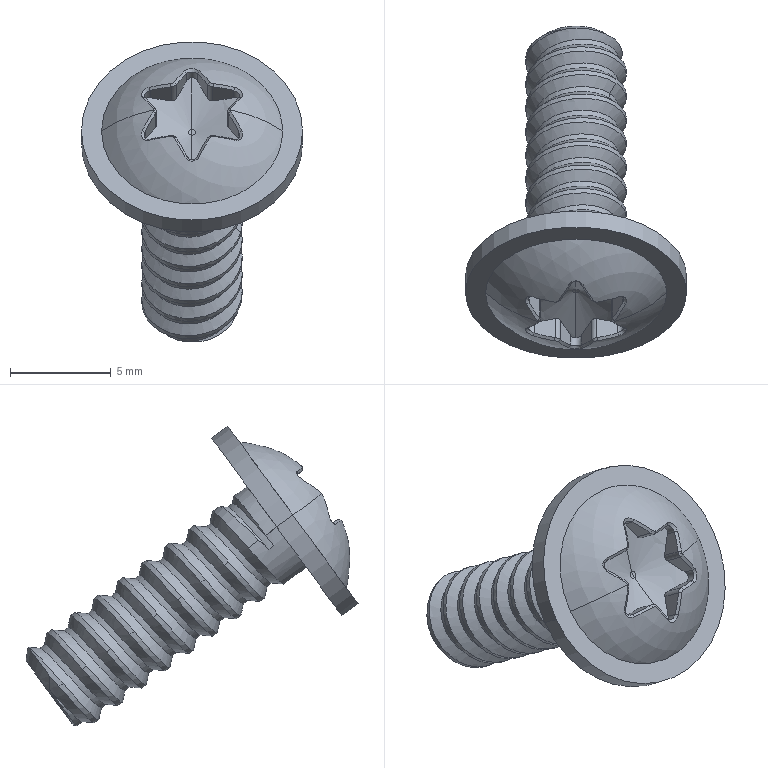Part | SolidWorks | features BaseBody 1 | 1 solid | 97 faces | box 11 x 16.533 x 14.92 mm | volume 379.358 mm3 | cylinder 35 | spline 26 | cone 17 | plane 15 | sphere 4 | commonest cylinder face diameters 5 x21 0.6 x12 11 x2